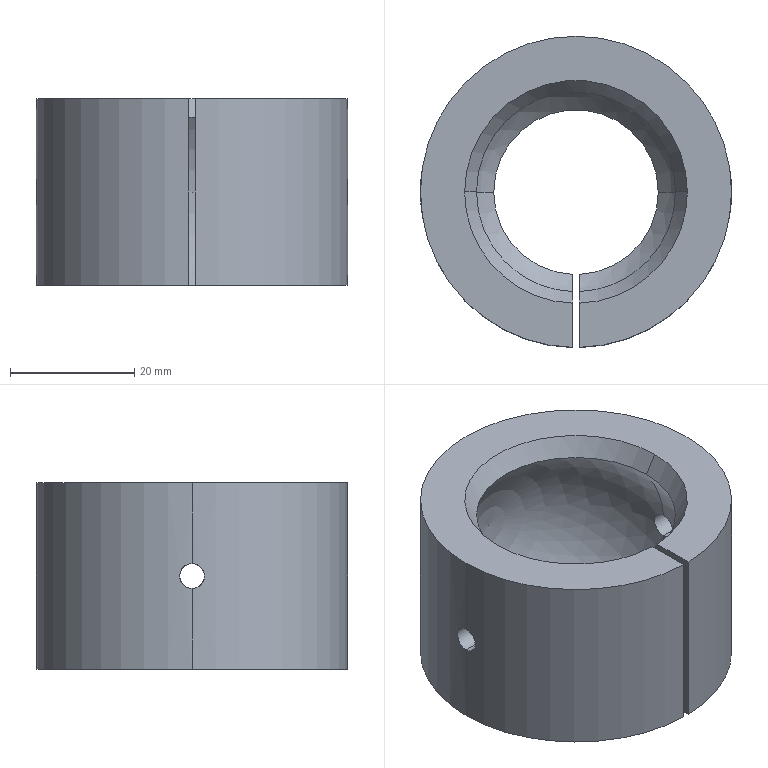Part | SolidWorks | features ICE 2, Revolution 1 | 1 solid | 17 faces | box 50 x 49.995 x 30 mm | volume 27277 mm3 | cylinder 7 | plane 4 | cone 3 | sphere 3 | commonest cylinder face diameters 4 x4 50 x3
STEP:
#1=CARTESIAN_POINT('',(19.9,0.,2.));
#2=VERTEX_POINT('',#1);
#3=CARTESIAN_POINT('',(19.9,0.,-2.));
#4=VERTEX_POINT('',#3);
#5=CARTESIAN_POINT('',(19.9,0.,0.));
#6=DIRECTION('',(1.,0.,0.));
#7=DIRECTION('',(0.,0.,1.));
#8=AXIS2_PLACEMENT_3D('',#5,#6,#7);
#9=CIRCLE('',#8,2.);
#10=EDGE_CURVE('',#2,#4,#9,.T.);
#11=ORIENTED_EDGE('',*,*,#10,.F.);
#12=CARTESIAN_POINT('',(25.,0.,2.));
#13=VERTEX_POINT('',#12);
#14=CARTESIAN_POINT('',(-25.,0.,2.));
#15=DIRECTION('',(1.,0.,0.));
#16=VECTOR('',#15,1000.);
#17=LINE('',#14,#16);
#18=EDGE_CURVE('',#2,#13,#17,.T.);
#19=ORIENTED_EDGE('',*,*,#18,.T.);
#20=CARTESIAN_POINT('',(25.,0.,-2.));
#21=VERTEX_POINT('',#20);
#22=CARTESIAN_POINT('',(25.,0.,-2.));
#23=CARTESIAN_POINT('',(25.,-0.1322,-2.));
#24=CARTESIAN_POINT('',(24.999,-0.2622,-1.987));
#25=CARTESIAN_POINT('',(24.995,-0.5179,-1.936));
#26=CARTESIAN_POINT('',(24.992,-0.6449,-1.898));
#27=CARTESIAN_POINT('',(24.985,-0.8871,-1.797));
#28=CARTESIAN_POINT('',(24.98,-1.002,-1.736));
#29=CARTESIAN_POINT('',(24.97,-1.219,-1.591));
#30=CARTESIAN_POINT('',(24.965,-1.322,-1.506));
#31=CARTESIAN_POINT('',(24.95,-1.599,-1.229));
#32=CARTESIAN_POINT('',(24.939,-1.748,-1.006));
#33=CARTESIAN_POINT('',(24.924,-1.947,-0.525));
#34=CARTESIAN_POINT('',(24.92,-2.,-0.2617));
#35=CARTESIAN_POINT('',(24.92,-2.,0.1298));
#36=CARTESIAN_POINT('',(24.921,-1.987,0.2623));
#37=CARTESIAN_POINT('',(24.925,-1.936,0.5189));
#38=CARTESIAN_POINT('',(24.928,-1.898,0.6436));
#39=CARTESIAN_POINT('',(24.935,-1.798,0.8858));
#40=CARTESIAN_POINT('',(24.94,-1.735,1.003));
#41=CARTESIAN_POINT('',(24.949,-1.59,1.22));
#42=CARTESIAN_POINT('',(24.955,-1.508,1.321));
#43=CARTESIAN_POINT('',(24.965,-1.321,1.507));
#44=CARTESIAN_POINT('',(24.97,-1.22,1.59));
#45=CARTESIAN_POINT('',(24.98,-1.003,1.735));
#46=CARTESIAN_POINT('',(24.985,-0.8865,1.798));
#47=CARTESIAN_POINT('',(24.992,-0.6442,1.898));
#48=CARTESIAN_POINT('',(24.995,-0.5195,1.936));
#49=CARTESIAN_POINT('',(24.999,-0.2632,1.987));
#50=CARTESIAN_POINT('',(25.,-0.1306,2.));
#51=CARTESIAN_POINT('',(25.,0.,2.));
#52=B_SPLINE_CURVE_WITH_KNOTS('',3,(#22,#23,#24,#25,#26,#27,#28,#29,#30,#31,#32,#33,#34,#35,#36,#37,#38,#39,#40,#41,#42,#43,#44,#45,#46,#47,#48,#49,#50,#51),.UNSPECIFIED.,.F.,.F.,(4,2,2,2,2,2,2,2,2,2,2,2,2,2,4),(0.,0.000391,0.0007819,0.001173,0.001564,0.002346,0.003128,0.003519,0.00391,0.004301,0.004692,0.005083,0.005473,0.005864,0.006255),.UNSPECIFIED.);
#53=EDGE_CURVE('',#21,#13,#52,.T.);
#54=ORIENTED_EDGE('',*,*,#53,.F.);
#55=CARTESIAN_POINT('',(-25.,0.,-2.));
#56=DIRECTION('',(1.,0.,0.));
#57=VECTOR('',#56,1000.);
#58=LINE('',#55,#57);
#59=EDGE_CURVE('',#4,#21,#58,.T.);
#60=ORIENTED_EDGE('',*,*,#59,.F.);
#61=EDGE_LOOP('',(#11,#19,#54,#60));
#62=FACE_OUTER_BOUND('',#61,.T.);
#63=CARTESIAN_POINT('',(-25.,0.,0.));
#64=DIRECTION('',(1.,0.,0.));
#65=DIRECTION('',(0.,0.,-1.));
#66=AXIS2_PLACEMENT_3D('',#63,#64,#65);
#67=CYLINDRICAL_SURFACE('',#66,2.);
#68=ADVANCED_FACE('',(#62),#67,.F.);
#69=CARTESIAN_POINT('',(-25.,0.,2.));
#70=VERTEX_POINT('',#69);
#71=CARTESIAN_POINT('',(-25.,0.,-2.));
#72=VERTEX_POINT('',#71);
#73=CARTESIAN_POINT('',(-25.,0.,2.));
#74=CARTESIAN_POINT('',(-25.,-0.2611,2.));
#75=CARTESIAN_POINT('',(-24.996,-0.5242,1.948));
#76=CARTESIAN_POINT('',(-24.981,-1.006,1.748));
#77=CARTESIAN_POINT('',(-24.97,-1.229,1.599));
#78=CARTESIAN_POINT('',(-24.955,-1.505,1.323));
#79=CARTESIAN_POINT('',(-24.949,-1.59,1.22));
#80=CARTESIAN_POINT('',(-24.94,-1.735,1.003));
#81=CARTESIAN_POINT('',(-24.935,-1.797,0.8882));
#82=CARTESIAN_POINT('',(-24.928,-1.897,0.6463));
#83=CARTESIAN_POINT('',(-24.925,-1.936,0.5191));
#84=CARTESIAN_POINT('',(-24.921,-1.987,0.2635));
#85=CARTESIAN_POINT('',(-24.92,-2.,0.1336));
#86=CARTESIAN_POINT('',(-24.92,-2.,-0.1304));
#87=CARTESIAN_POINT('',(-24.921,-1.987,-0.2607));
#88=CARTESIAN_POINT('',(-24.925,-1.937,-0.5164));
#89=CARTESIAN_POINT('',(-24.928,-1.898,-0.6433));
#90=CARTESIAN_POINT('',(-24.935,-1.798,-0.8857));
#91=CARTESIAN_POINT('',(-24.94,-1.737,-1.001));
#92=CARTESIAN_POINT('',(-24.949,-1.592,-1.218));
#93=CARTESIAN_POINT('',(-24.955,-1.507,-1.321));
#94=CARTESIAN_POINT('',(-24.97,-1.231,-1.598));
#95=CARTESIAN_POINT('',(-24.981,-1.008,-1.747));
#96=CARTESIAN_POINT('',(-24.996,-0.527,-1.947));
#97=CARTESIAN_POINT('',(-25.,-0.2643,-2.));
#98=CARTESIAN_POINT('',(-25.,0.,-2.));
#99=B_SPLINE_CURVE_WITH_KNOTS('',3,(#73,#74,#75,#76,#77,#78,#79,#80,#81,#82,#83,#84,#85,#86,#87,#88,#89,#90,#91,#92,#93,#94,#95,#96,#97,#98),.UNSPECIFIED.,.F.,.F.,(4,2,2,2,2,2,2,2,2,2,2,2,4),(0.006255,0.007037,0.007819,0.00821,0.008601,0.008992,0.009382,0.009773,0.01016,0.01056,0.01095,0.01173,0.01251),.UNSPECIFIED.);
#100=EDGE_CURVE('',#70,#72,#99,.T.);
#101=ORIENTED_EDGE('',*,*,#100,.F.);
#102=CARTESIAN_POINT('',(-19.9,0.,2.));
#103=VERTEX_POINT('',#102);
#104=CARTESIAN_POINT('',(-25.,0.,2.));
#105=DIRECTION('',(1.,0.,0.));
#106=VECTOR('',#105,1000.);
#107=LINE('',#104,#106);
#108=EDGE_CURVE('',#70,#103,#107,.T.);
#109=ORIENTED_EDGE('',*,*,#108,.T.);
#110=CARTESIAN_POINT('',(-19.9,0.,-2.));
#111=VERTEX_POINT('',#110);
#112=CARTESIAN_POINT('',(-19.9,0.,0.));
#113=DIRECTION('',(-1.,0.,0.));
#114=DIRECTION('',(0.,0.,-1.));
#115=AXIS2_PLACEMENT_3D('',#112,#113,#114);
#116=CIRCLE('',#115,2.);
#117=EDGE_CURVE('',#111,#103,#116,.T.);
#118=ORIENTED_EDGE('',*,*,#117,.F.);
#119=CARTESIAN_POINT('',(-25.,0.,-2.));
#120=DIRECTION('',(1.,0.,0.));
#121=VECTOR('',#120,1000.);
#122=LINE('',#119,#121);
#123=EDGE_CURVE('',#72,#111,#122,.T.);
#124=ORIENTED_EDGE('',*,*,#123,.F.);
#125=EDGE_LOOP('',(#101,#109,#118,#124));
#126=FACE_OUTER_BOUND('',#125,.T.);
#127=CARTESIAN_POINT('',(-25.,0.,0.));
#128=DIRECTION('',(1.,0.,0.));
#129=DIRECTION('',(0.,0.,-1.));
#130=AXIS2_PLACEMENT_3D('',#127,#128,#129);
#131=CYLINDRICAL_SURFACE('',#130,2.);
#132=ADVANCED_FACE('',(#126),#131,.F.);
#133=CARTESIAN_POINT('',(-0.5,-15.992,12.));
#134=VERTEX_POINT('',#133);
#135=CARTESIAN_POINT('',(-16.,0.,12.));
#136=VERTEX_POINT('',#135);
#137=CARTESIAN_POINT('',(0.,0.,12.));
#138=DIRECTION('',(0.,0.,-1.));
#139=DIRECTION('',(-1.,0.,0.));
#140=AXIS2_PLACEMENT_3D('',#137,#138,#139);
#141=CIRCLE('',#140,16.);
#142=EDGE_CURVE('',#134,#136,#141,.T.);
#143=ORIENTED_EDGE('',*,*,#142,.T.);
#144=CARTESIAN_POINT('',(-17.9,0.,15.));
#145=VERTEX_POINT('',#144);
#146=CARTESIAN_POINT('',(-16.,0.,12.));
#147=DIRECTION('',(-0.5351,0.,0.8448));
#148=VECTOR('',#147,1000.);
#149=LINE('',#146,#148);
#150=EDGE_CURVE('',#136,#145,#149,.T.);
#151=ORIENTED_EDGE('',*,*,#150,.T.);
#152=CARTESIAN_POINT('',(-0.5,-17.893,15.));
#153=VERTEX_POINT('',#152);
#154=CARTESIAN_POINT('',(0.,0.,15.));
#155=DIRECTION('',(0.,0.,-1.));
#156=DIRECTION('',(-1.,0.,0.));
#157=AXIS2_PLACEMENT_3D('',#154,#155,#156);
#158=CIRCLE('',#157,17.9);
#159=EDGE_CURVE('',#153,#145,#158,.T.);
#160=ORIENTED_EDGE('',*,*,#159,.F.);
#161=CARTESIAN_POINT('',(-0.5,-17.893,15.));
#162=CARTESIAN_POINT('',(-0.5,-17.259,14.));
#163=CARTESIAN_POINT('',(-0.5,-16.626,13.));
#164=CARTESIAN_POINT('',(-0.5,-15.992,12.));
#165=B_SPLINE_CURVE_WITH_KNOTS('',3,(#161,#162,#163,#164),.UNSPECIFIED.,.F.,.F.,(4,4),(0.01915,0.0227),.UNSPECIFIED.);
#166=EDGE_CURVE('',#153,#134,#165,.T.);
#167=ORIENTED_EDGE('',*,*,#166,.T.);
#168=EDGE_LOOP('',(#143,#151,#160,#167));
#169=FACE_OUTER_BOUND('',#168,.T.);
#170=CARTESIAN_POINT('',(0.,0.,12.));
#171=DIRECTION('',(0.,0.,1.));
#172=DIRECTION('',(1.,0.,0.));
#173=AXIS2_PLACEMENT_3D('',#170,#171,#172);
#174=CONICAL_SURFACE('',#173,16.,0.5646);
#175=ADVANCED_FACE('',(#169),#174,.F.);
#176=ORIENTED_EDGE('',*,*,#150,.F.);
#177=CARTESIAN_POINT('',(16.,0.,12.));
#178=VERTEX_POINT('',#177);
#179=CARTESIAN_POINT('',(0.,0.,12.));
#180=DIRECTION('',(0.,0.,-1.));
#181=DIRECTION('',(-1.,0.,0.));
#182=AXIS2_PLACEMENT_3D('',#179,#180,#181);
#183=CIRCLE('',#182,16.);
#184=EDGE_CURVE('',#136,#178,#183,.T.);
#185=ORIENTED_EDGE('',*,*,#184,.T.);
#186=CARTESIAN_POINT('',(17.9,0.,15.));
#187=VERTEX_POINT('',#186);
#188=CARTESIAN_POINT('',(16.,0.,12.));
#189=DIRECTION('',(0.5351,0.,0.8448));
#190=VECTOR('',#189,1000.);
#191=LINE('',#188,#190);
#192=EDGE_CURVE('',#178,#187,#191,.T.);
#193=ORIENTED_EDGE('',*,*,#192,.T.);
#194=CARTESIAN_POINT('',(0.,0.,15.));
#195=DIRECTION('',(0.,0.,-1.));
#196=DIRECTION('',(-1.,0.,0.));
#197=AXIS2_PLACEMENT_3D('',#194,#195,#196);
#198=CIRCLE('',#197,17.9);
#199=EDGE_CURVE('',#145,#187,#198,.T.);
#200=ORIENTED_EDGE('',*,*,#199,.F.);
#201=EDGE_LOOP('',(#176,#185,#193,#200));
#202=FACE_OUTER_BOUND('',#201,.T.);
#203=CARTESIAN_POINT('',(0.,0.,12.));
#204=DIRECTION('',(0.,0.,1.));
#205=DIRECTION('',(1.,0.,0.));
#206=AXIS2_PLACEMENT_3D('',#203,#204,#205);
#207=CONICAL_SURFACE('',#206,16.,0.5646);
#208=ADVANCED_FACE('',(#202),#207,.F.);
#209=ORIENTED_EDGE('',*,*,#184,.F.);
#210=CARTESIAN_POINT('',(0.,0.,0.));
#211=DIRECTION('',(0.,-1.,0.));
#212=DIRECTION('',(1.,0.,0.));
#213=AXIS2_PLACEMENT_3D('',#210,#211,#212);
#214=CIRCLE('',#213,20.);
#215=EDGE_CURVE('',#136,#103,#214,.T.);
#216=ORIENTED_EDGE('',*,*,#215,.T.);
#217=CARTESIAN_POINT('',(-19.9,0.,0.));
#218=DIRECTION('',(-1.,0.,0.));
#219=DIRECTION('',(0.,0.,-1.));
#220=AXIS2_PLACEMENT_3D('',#217,#218,#219);
#221=CIRCLE('',#220,2.);
#222=EDGE_CURVE('',#103,#111,#221,.T.);
#223=ORIENTED_EDGE('',*,*,#222,.T.);
#224=CARTESIAN_POINT('',(-13.229,0.,-15.));
#225=VERTEX_POINT('',#224);
#226=CARTESIAN_POINT('',(0.,0.,0.));
#227=DIRECTION('',(0.,-1.,0.));
#228=DIRECTION('',(1.,0.,0.));
#229=AXIS2_PLACEMENT_3D('',#226,#227,#228);
#230=CIRCLE('',#229,20.);
#231=EDGE_CURVE('',#111,#225,#230,.T.);
#232=ORIENTED_EDGE('',*,*,#231,.T.);
#233=CARTESIAN_POINT('',(13.229,0.,-15.));
#234=VERTEX_POINT('',#233);
#235=CARTESIAN_POINT('',(0.,0.,-15.));
#236=DIRECTION('',(0.,0.,-1.));
#237=DIRECTION('',(-1.,0.,0.));
#238=AXIS2_PLACEMENT_3D('',#235,#236,#237);
#239=CIRCLE('',#238,13.229);
#240=EDGE_CURVE('',#225,#234,#239,.T.);
#241=ORIENTED_EDGE('',*,*,#240,.T.);
#242=CARTESIAN_POINT('',(0.,0.,0.));
#243=DIRECTION('',(0.,1.,0.));
#244=DIRECTION('',(0.,0.,1.));
#245=AXIS2_PLACEMENT_3D('',#242,#243,#244);
#246=CIRCLE('',#245,20.);
#247=EDGE_CURVE('',#4,#234,#246,.T.);
#248=ORIENTED_EDGE('',*,*,#247,.F.);
#249=CARTESIAN_POINT('',(19.9,0.,0.));
#250=DIRECTION('',(1.,0.,0.));
#251=DIRECTION('',(0.,0.,1.));
#252=AXIS2_PLACEMENT_3D('',#249,#250,#251);
#253=CIRCLE('',#252,2.);
#254=EDGE_CURVE('',#4,#2,#253,.T.);
#255=ORIENTED_EDGE('',*,*,#254,.T.);
#256=CARTESIAN_POINT('',(0.,0.,0.));
#257=DIRECTION('',(0.,1.,0.));
#258=DIRECTION('',(0.,0.,1.));
#259=AXIS2_PLACEMENT_3D('',#256,#257,#258);
#260=CIRCLE('',#259,20.);
#261=EDGE_CURVE('',#178,#2,#260,.T.);
#262=ORIENTED_EDGE('',*,*,#261,.F.);
#263=EDGE_LOOP('',(#209,#216,#223,#232,#241,#248,#255,#262));
#264=FACE_OUTER_BOUND('',#263,.T.);
#265=CARTESIAN_POINT('',(0.,0.,0.));
#266=DIRECTION('',(0.,-1.,0.));
#267=DIRECTION('',(1.,0.,0.));
#268=AXIS2_PLACEMENT_3D('',#265,#266,#267);
#269=SPHERICAL_SURFACE('',#268,20.);
#270=ADVANCED_FACE('',(#264),#269,.F.);
#271=CARTESIAN_POINT('',(0.5,-15.992,12.));
#272=VERTEX_POINT('',#271);
#273=CARTESIAN_POINT('',(0.,0.,12.));
#274=DIRECTION('',(0.,0.,-1.));
#275=DIRECTION('',(-1.,0.,0.));
#276=AXIS2_PLACEMENT_3D('',#273,#274,#275);
#277=CIRCLE('',#276,16.);
#278=EDGE_CURVE('',#178,#272,#277,.T.);
#279=ORIENTED_EDGE('',*,*,#278,.F.);
#280=ORIENTED_EDGE('',*,*,#261,.T.);
#281=ORIENTED_EDGE('',*,*,#10,.T.);
#282=ORIENTED_EDGE('',*,*,#247,.T.);
#283=CARTESIAN_POINT('',(0.5,-13.219,-15.));
#284=VERTEX_POINT('',#283);
#285=CARTESIAN_POINT('',(0.,0.,-15.));
#286=DIRECTION('',(0.,0.,-1.));
#287=DIRECTION('',(-1.,0.,0.));
#288=AXIS2_PLACEMENT_3D('',#285,#286,#287);
#289=CIRCLE('',#288,13.229);
#290=EDGE_CURVE('',#234,#284,#289,.T.);
#291=ORIENTED_EDGE('',*,*,#290,.T.);
#292=CARTESIAN_POINT('',(0.5,0.,0.));
#293=DIRECTION('',(-1.,0.,0.));
#294=DIRECTION('',(0.,0.,-1.));
#295=AXIS2_PLACEMENT_3D('',#292,#293,#294);
#296=CIRCLE('',#295,19.994);
#297=EDGE_CURVE('',#284,#272,#296,.T.);
#298=ORIENTED_EDGE('',*,*,#297,.T.);
#299=EDGE_LOOP('',(#279,#280,#281,#282,#291,#298));
#300=FACE_OUTER_BOUND('',#299,.T.);
#301=CARTESIAN_POINT('',(0.,0.,0.));
#302=DIRECTION('',(0.,-1.,0.));
#303=DIRECTION('',(1.,0.,0.));
#304=AXIS2_PLACEMENT_3D('',#301,#302,#303);
#305=SPHERICAL_SURFACE('',#304,20.);
#306=ADVANCED_FACE('',(#300),#305,.F.);
#307=CARTESIAN_POINT('',(-25.,0.,15.));
#308=VERTEX_POINT('',#307);
#309=CARTESIAN_POINT('',(25.,0.,15.));
#310=VERTEX_POINT('',#309);
#311=CARTESIAN_POINT('',(0.,0.,15.));
#312=DIRECTION('',(0.,0.,-1.));
#313=DIRECTION('',(-1.,0.,0.));
#314=AXIS2_PLACEMENT_3D('',#311,#312,#313);
#315=CIRCLE('',#314,25.);
#316=EDGE_CURVE('',#308,#310,#315,.T.);
#317=ORIENTED_EDGE('',*,*,#316,.T.);
#318=CARTESIAN_POINT('',(25.,0.,-23.629));
#319=DIRECTION('',(0.,0.,-1.));
#320=VECTOR('',#319,1000.);
#321=LINE('',#318,#320);
#322=EDGE_CURVE('',#310,#13,#321,.T.);
#323=ORIENTED_EDGE('',*,*,#322,.T.);
#324=CARTESIAN_POINT('',(25.,0.,2.));
#325=CARTESIAN_POINT('',(25.,0.2611,2.));
#326=CARTESIAN_POINT('',(24.996,0.5242,1.948));
#327=CARTESIAN_POINT('',(24.981,1.006,1.748));
#328=CARTESIAN_POINT('',(24.97,1.229,1.599));
#329=CARTESIAN_POINT('',(24.955,1.505,1.323));
#330=CARTESIAN_POINT('',(24.949,1.59,1.22));
#331=CARTESIAN_POINT('',(24.94,1.735,1.003));
#332=CARTESIAN_POINT('',(24.935,1.797,0.8882));
#333=CARTESIAN_POINT('',(24.928,1.897,0.6463));
#334=CARTESIAN_POINT('',(24.925,1.936,0.5191));
#335=CARTESIAN_POINT('',(24.921,1.987,0.2635));
#336=CARTESIAN_POINT('',(24.92,2.,0.1336));
#337=CARTESIAN_POINT('',(24.92,2.,-0.1304));
#338=CARTESIAN_POINT('',(24.921,1.987,-0.2607));
#339=CARTESIAN_POINT('',(24.925,1.937,-0.5164));
#340=CARTESIAN_POINT('',(24.928,1.898,-0.6433));
#341=CARTESIAN_POINT('',(24.935,1.798,-0.8857));
#342=CARTESIAN_POINT('',(24.94,1.737,-1.001));
#343=CARTESIAN_POINT('',(24.949,1.592,-1.218));
#344=CARTESIAN_POINT('',(24.955,1.507,-1.321));
#345=CARTESIAN_POINT('',(24.97,1.231,-1.598));
#346=CARTESIAN_POINT('',(24.981,1.008,-1.747));
#347=CARTESIAN_POINT('',(24.996,0.527,-1.947));
#348=CARTESIAN_POINT('',(25.,0.2643,-2.));
#349=CARTESIAN_POINT('',(25.,0.,-2.));
#350=B_SPLINE_CURVE_WITH_KNOTS('',3,(#324,#325,#326,#327,#328,#329,#330,#331,#332,#333,#334,#335,#336,#337,#338,#339,#340,#341,#342,#343,#344,#345,#346,#347,#348,#349),.UNSPECIFIED.,.F.,.F.,(4,2,2,2,2,2,2,2,2,2,2,2,4),(0.006255,0.007037,0.007819,0.00821,0.008601,0.008992,0.009382,0.009773,0.01016,0.01056,0.01095,0.01173,0.01251),.UNSPECIFIED.);
#351=EDGE_CURVE('',#13,#21,#350,.T.);
#352=ORIENTED_EDGE('',*,*,#351,.T.);
#353=CARTESIAN_POINT('',(25.,0.,-15.));
#354=VERTEX_POINT('',#353);
#355=CARTESIAN_POINT('',(25.,0.,-23.629));
#356=DIRECTION('',(0.,0.,-1.));
#357=VECTOR('',#356,1000.);
#358=LINE('',#355,#357);
#359=EDGE_CURVE('',#21,#354,#358,.T.);
#360=ORIENTED_EDGE('',*,*,#359,.T.);
#361=CARTESIAN_POINT('',(-25.,0.,-15.));
#362=VERTEX_POINT('',#361);
#363=CARTESIAN_POINT('',(0.,0.,-15.));
#364=DIRECTION('',(0.,0.,-1.));
#365=DIRECTION('',(-1.,0.,0.));
#366=AXIS2_PLACEMENT_3D('',#363,#364,#365);
#367=CIRCLE('',#366,25.);
#368=EDGE_CURVE('',#362,#354,#367,.T.);
#369=ORIENTED_EDGE('',*,*,#368,.F.);
#370=CARTESIAN_POINT('',(-25.,0.,-23.629));
#371=DIRECTION('',(0.,0.,-1.));
#372=VECTOR('',#371,1000.);
#373=LINE('',#370,#372);
#374=EDGE_CURVE('',#72,#362,#373,.T.);
#375=ORIENTED_EDGE('',*,*,#374,.F.);
#376=CARTESIAN_POINT('',(-25.,0.,-2.));
#377=CARTESIAN_POINT('',(-25.,0.1322,-2.));
#378=CARTESIAN_POINT('',(-24.999,0.2622,-1.987));
#379=CARTESIAN_POINT('',(-24.995,0.5179,-1.936));
#380=CARTESIAN_POINT('',(-24.992,0.6449,-1.898));
#381=CARTESIAN_POINT('',(-24.985,0.8871,-1.797));
#382=CARTESIAN_POINT('',(-24.98,1.002,-1.736));
#383=CARTESIAN_POINT('',(-24.97,1.219,-1.591));
#384=CARTESIAN_POINT('',(-24.965,1.322,-1.506));
#385=CARTESIAN_POINT('',(-24.95,1.599,-1.229));
#386=CARTESIAN_POINT('',(-24.939,1.748,-1.006));
#387=CARTESIAN_POINT('',(-24.924,1.947,-0.525));
#388=CARTESIAN_POINT('',(-24.92,2.,-0.2617));
#389=CARTESIAN_POINT('',(-24.92,2.,0.1298));
#390=CARTESIAN_POINT('',(-24.921,1.987,0.2623));
#391=CARTESIAN_POINT('',(-24.925,1.936,0.5189));
#392=CARTESIAN_POINT('',(-24.928,1.898,0.6436));
#393=CARTESIAN_POINT('',(-24.935,1.798,0.8858));
#394=CARTESIAN_POINT('',(-24.94,1.735,1.003));
#395=CARTESIAN_POINT('',(-24.949,1.59,1.22));
#396=CARTESIAN_POINT('',(-24.955,1.508,1.321));
#397=CARTESIAN_POINT('',(-24.965,1.321,1.507));
#398=CARTESIAN_POINT('',(-24.97,1.22,1.59));
#399=CARTESIAN_POINT('',(-24.98,1.003,1.735));
#400=CARTESIAN_POINT('',(-24.985,0.8865,1.798));
#401=CARTESIAN_POINT('',(-24.992,0.6442,1.898));
#402=CARTESIAN_POINT('',(-24.995,0.5195,1.936));
#403=CARTESIAN_POINT('',(-24.999,0.2632,1.987));
#404=CARTESIAN_POINT('',(-25.,0.1306,2.));
#405=CARTESIAN_POINT('',(-25.,0.,2.));
#406=B_SPLINE_CURVE_WITH_KNOTS('',3,(#376,#377,#378,#379,#380,#381,#382,#383,#384,#385,#386,#387,#388,#389,#390,#391,#392,#393,#394,#395,#396,#397,#398,#399,#400,#401,#402,#403,#404,#405),.UNSPECIFIED.,.F.,.F.,(4,2,2,2,2,2,2,2,2,2,2,2,2,2,4),(0.,0.000391,0.0007819,0.001173,0.001564,0.002346,0.003128,0.003519,0.00391,0.004301,0.004692,0.005083,0.005473,0.005864,0.006255),.UNSPECIFIED.);
#407=EDGE_CURVE('',#72,#70,#406,.T.);
#408=ORIENTED_EDGE('',*,*,#407,.T.);
#409=CARTESIAN_POINT('',(-25.,0.,-23.629));
#410=DIRECTION('',(0.,0.,-1.));
#411=VECTOR('',#410,1000.);
#412=LINE('',#409,#411);
#413=EDGE_CURVE('',#308,#70,#412,.T.);
#414=ORIENTED_EDGE('',*,*,#413,.F.);
#415=EDGE_LOOP('',(#317,#323,#352,#360,#369,#375,#408,#414));
#416=FACE_OUTER_BOUND('',#415,.T.);
#417=CARTESIAN_POINT('',(0.,0.,-23.629));
#418=DIRECTION('',(0.,0.,-1.));
#419=DIRECTION('',(-1.,0.,0.));
#420=AXIS2_PLACEMENT_3D('',#417,#418,#419);
#421=CYLINDRICAL_SURFACE('',#420,25.);
#422=ADVANCED_FACE('',(#416),#421,.T.);
#423=CARTESIAN_POINT('',(-0.5,-24.995,15.));
#424=VERTEX_POINT('',#423);
#425=CARTESIAN_POINT('',(0.,0.,15.));
#426=DIRECTION('',(0.,0.,-1.));
#427=DIRECTION('',(-1.,0.,0.));
#428=AXIS2_PLACEMENT_3D('',#425,#426,#427);
#429=CIRCLE('',#428,25.);
#430=EDGE_CURVE('',#424,#308,#429,.T.);
#431=ORIENTED_EDGE('',*,*,#430,.T.);
#432=ORIENTED_EDGE('',*,*,#413,.T.);
#433=ORIENTED_EDGE('',*,*,#100,.T.);
#434=ORIENTED_EDGE('',*,*,#374,.T.);
#435=CARTESIAN_POINT('',(-0.5,-24.995,-15.));
#436=VERTEX_POINT('',#435);
#437=CARTESIAN_POINT('',(0.,0.,-15.));
#438=DIRECTION('',(0.,0.,-1.));
#439=DIRECTION('',(-1.,0.,0.));
#440=AXIS2_PLACEMENT_3D('',#437,#438,#439);
#441=CIRCLE('',#440,25.);
#442=EDGE_CURVE('',#436,#362,#441,.T.);
#443=ORIENTED_EDGE('',*,*,#442,.F.);
#444=CARTESIAN_POINT('',(-0.5,-24.995,-23.629));
#445=DIRECTION('',(0.,0.,1.));
#446=VECTOR('',#445,1000.);
#447=LINE('',#444,#446);
#448=EDGE_CURVE('',#436,#424,#447,.T.);
#449=ORIENTED_EDGE('',*,*,#448,.T.);
#450=EDGE_LOOP('',(#431,#432,#433,#434,#443,#449));
#451=FACE_OUTER_BOUND('',#450,.T.);
#452=CARTESIAN_POINT('',(0.,0.,-23.629));
#453=DIRECTION('',(0.,0.,-1.));
#454=DIRECTION('',(-1.,0.,0.));
#455=AXIS2_PLACEMENT_3D('',#452,#453,#454);
#456=CYLINDRICAL_SURFACE('',#455,25.);
#457=ADVANCED_FACE('',(#451),#456,.T.);
#458=ORIENTED_EDGE('',*,*,#322,.F.);
#459=CARTESIAN_POINT('',(0.5,-24.995,15.));
#460=VERTEX_POINT('',#459);
#461=CARTESIAN_POINT('',(0.,0.,15.));
#462=DIRECTION('',(0.,0.,-1.));
#463=DIRECTION('',(-1.,0.,0.));
#464=AXIS2_PLACEMENT_3D('',#461,#462,#463);
#465=CIRCLE('',#464,25.);
#466=EDGE_CURVE('',#310,#460,#465,.T.);
#467=ORIENTED_EDGE('',*,*,#466,.T.);
#468=CARTESIAN_POINT('',(0.5,-24.995,-15.));
#469=VERTEX_POINT('',#468);
#470=CARTESIAN_POINT('',(0.5,-24.995,-23.629));
#471=DIRECTION('',(0.,0.,-1.));
#472=VECTOR('',#471,1000.);
#473=LINE('',#470,#472);
#474=EDGE_CURVE('',#460,#469,#473,.T.);
#475=ORIENTED_EDGE('',*,*,#474,.T.);
#476=CARTESIAN_POINT('',(0.,0.,-15.));
#477=DIRECTION('',(0.,0.,-1.));
#478=DIRECTION('',(-1.,0.,0.));
#479=AXIS2_PLACEMENT_3D('',#476,#477,#478);
#480=CIRCLE('',#479,25.);
#481=EDGE_CURVE('',#354,#469,#480,.T.);
#482=ORIENTED_EDGE('',*,*,#481,.F.);
#483=ORIENTED_EDGE('',*,*,#359,.F.);
#484=ORIENTED_EDGE('',*,*,#53,.T.);
#485=EDGE_LOOP('',(#458,#467,#475,#482,#483,#484));
#486=FACE_OUTER_BOUND('',#485,.T.);
#487=CARTESIAN_POINT('',(0.,0.,-23.629));
#488=DIRECTION('',(0.,0.,-1.));
#489=DIRECTION('',(-1.,0.,0.));
#490=AXIS2_PLACEMENT_3D('',#487,#488,#489);
#491=CYLINDRICAL_SURFACE('',#490,25.);
#492=ADVANCED_FACE('',(#486),#491,.T.);
#493=CARTESIAN_POINT('',(-0.5,-13.219,-15.));
#494=VERTEX_POINT('',#493);
#495=CARTESIAN_POINT('',(0.,0.,-15.));
#496=DIRECTION('',(0.,0.,-1.));
#497=DIRECTION('',(-1.,0.,0.));
#498=AXIS2_PLACEMENT_3D('',#495,#496,#497);
#499=CIRCLE('',#498,13.229);
#500=EDGE_CURVE('',#494,#225,#499,.T.);
#501=ORIENTED_EDGE('',*,*,#500,.F.);
#502=CARTESIAN_POINT('',(-0.5,0.,-15.));
#503=DIRECTION('',(0.,-1.,0.));
#504=VECTOR('',#503,1000.);
#505=LINE('',#502,#504);
#506=EDGE_CURVE('',#494,#436,#505,.T.);
#507=ORIENTED_EDGE('',*,*,#506,.T.);
#508=ORIENTED_EDGE('',*,*,#442,.T.);
#509=ORIENTED_EDGE('',*,*,#368,.T.);
#510=ORIENTED_EDGE('',*,*,#481,.T.);
#511=CARTESIAN_POINT('',(0.5,0.,-15.));
#512=DIRECTION('',(0.,1.,0.));
#513=VECTOR('',#512,1000.);
#514=LINE('',#511,#513);
#515=EDGE_CURVE('',#469,#284,#514,.T.);
#516=ORIENTED_EDGE('',*,*,#515,.T.);
#517=ORIENTED_EDGE('',*,*,#290,.F.);
#518=ORIENTED_EDGE('',*,*,#240,.F.);
#519=EDGE_LOOP('',(#501,#507,#508,#509,#510,#516,#517,#518));
#520=FACE_OUTER_BOUND('',#519,.T.);
#521=CARTESIAN_POINT('',(13.229,0.,-15.));
#522=DIRECTION('',(0.,0.,1.));
#523=DIRECTION('',(1.,0.,0.));
#524=AXIS2_PLACEMENT_3D('',#521,#522,#523);
#525=PLANE('',#524);
#526=ADVANCED_FACE('',(#520),#525,.F.);
#527=ORIENTED_EDGE('',*,*,#215,.F.);
#528=ORIENTED_EDGE('',*,*,#142,.F.);
#529=CARTESIAN_POINT('',(-0.5,0.,0.));
#530=DIRECTION('',(1.,0.,0.));
#531=DIRECTION('',(0.,0.,1.));
#532=AXIS2_PLACEMENT_3D('',#529,#530,#531);
#533=CIRCLE('',#532,19.994);
#534=EDGE_CURVE('',#134,#494,#533,.T.);
#535=ORIENTED_EDGE('',*,*,#534,.T.);
#536=ORIENTED_EDGE('',*,*,#500,.T.);
#537=ORIENTED_EDGE('',*,*,#231,.F.);
#538=ORIENTED_EDGE('',*,*,#117,.T.);
#539=EDGE_LOOP('',(#527,#528,#535,#536,#537,#538));
#540=FACE_OUTER_BOUND('',#539,.T.);
#541=CARTESIAN_POINT('',(0.,0.,0.));
#542=DIRECTION('',(0.,-1.,0.));
#543=DIRECTION('',(1.,0.,0.));
#544=AXIS2_PLACEMENT_3D('',#541,#542,#543);
#545=SPHERICAL_SURFACE('',#544,20.);
#546=ADVANCED_FACE('',(#540),#545,.F.);
#547=ORIENTED_EDGE('',*,*,#192,.F.);
#548=ORIENTED_EDGE('',*,*,#278,.T.);
#549=CARTESIAN_POINT('',(0.5,-17.893,15.));
#550=VERTEX_POINT('',#549);
#551=CARTESIAN_POINT('',(0.5,-15.992,12.));
#552=CARTESIAN_POINT('',(0.5,-16.187,12.307));
#553=CARTESIAN_POINT('',(0.5,-16.381,12.614));
#554=CARTESIAN_POINT('',(0.5,-16.576,12.921));
#555=CARTESIAN_POINT('',(0.5,-17.015,13.614));
#556=CARTESIAN_POINT('',(0.5,-17.454,14.307));
#557=CARTESIAN_POINT('',(0.5,-17.893,15.));
#558=B_SPLINE_CURVE_WITH_KNOTS('',3,(#551,#552,#553,#554,#555,#556,#557),.UNSPECIFIED.,.F.,.F.,(4,3,4),(0.02052,0.02161,0.02407),.UNSPECIFIED.);
#559=EDGE_CURVE('',#272,#550,#558,.T.);
#560=ORIENTED_EDGE('',*,*,#559,.T.);
#561=CARTESIAN_POINT('',(0.,0.,15.));
#562=DIRECTION('',(0.,0.,-1.));
#563=DIRECTION('',(-1.,0.,0.));
#564=AXIS2_PLACEMENT_3D('',#561,#562,#563);
#565=CIRCLE('',#564,17.9);
#566=EDGE_CURVE('',#187,#550,#565,.T.);
#567=ORIENTED_EDGE('',*,*,#566,.F.);
#568=EDGE_LOOP('',(#547,#548,#560,#567));
#569=FACE_OUTER_BOUND('',#568,.T.);
#570=CARTESIAN_POINT('',(0.,0.,12.));
#571=DIRECTION('',(0.,0.,1.));
#572=DIRECTION('',(1.,0.,0.));
#573=AXIS2_PLACEMENT_3D('',#570,#571,#572);
#574=CONICAL_SURFACE('',#573,16.,0.5646);
#575=ADVANCED_FACE('',(#569),#574,.F.);
#576=ORIENTED_EDGE('',*,*,#430,.F.);
#577=CARTESIAN_POINT('',(-0.5,0.,15.));
#578=DIRECTION('',(0.,1.,0.));
#579=VECTOR('',#578,1000.);
#580=LINE('',#577,#579);
#581=EDGE_CURVE('',#424,#153,#580,.T.);
#582=ORIENTED_EDGE('',*,*,#581,.T.);
#583=ORIENTED_EDGE('',*,*,#159,.T.);
#584=ORIENTED_EDGE('',*,*,#199,.T.);
#585=ORIENTED_EDGE('',*,*,#566,.T.);
#586=CARTESIAN_POINT('',(0.5,0.,15.));
#587=DIRECTION('',(0.,-1.,0.));
#588=VECTOR('',#587,1000.);
#589=LINE('',#586,#588);
#590=EDGE_CURVE('',#550,#460,#589,.T.);
#591=ORIENTED_EDGE('',*,*,#590,.T.);
#592=ORIENTED_EDGE('',*,*,#466,.F.);
#593=ORIENTED_EDGE('',*,*,#316,.F.);
#594=EDGE_LOOP('',(#576,#582,#583,#584,#585,#591,#592,#593));
#595=FACE_OUTER_BOUND('',#594,.T.);
#596=CARTESIAN_POINT('',(17.9,0.,15.));
#597=DIRECTION('',(0.,0.,-1.));
#598=DIRECTION('',(-1.,0.,0.));
#599=AXIS2_PLACEMENT_3D('',#596,#597,#598);
#600=PLANE('',#599);
#601=ADVANCED_FACE('',(#595),#600,.F.);
#602=ORIENTED_EDGE('',*,*,#590,.F.);
#603=ORIENTED_EDGE('',*,*,#559,.F.);
#604=ORIENTED_EDGE('',*,*,#297,.F.);
#605=ORIENTED_EDGE('',*,*,#515,.F.);
#606=ORIENTED_EDGE('',*,*,#474,.F.);
#607=EDGE_LOOP('',(#602,#603,#604,#605,#606));
#608=FACE_OUTER_BOUND('',#607,.T.);
#609=CARTESIAN_POINT('',(0.5,-25.,-17.5));
#610=DIRECTION('',(1.,0.,0.));
#611=DIRECTION('',(0.,0.,-1.));
#612=AXIS2_PLACEMENT_3D('',#609,#610,#611);
#613=PLANE('',#612);
#614=ADVANCED_FACE('',(#608),#613,.F.);
#615=ORIENTED_EDGE('',*,*,#506,.F.);
#616=ORIENTED_EDGE('',*,*,#534,.F.);
#617=ORIENTED_EDGE('',*,*,#166,.F.);
#618=ORIENTED_EDGE('',*,*,#581,.F.);
#619=ORIENTED_EDGE('',*,*,#448,.F.);
#620=EDGE_LOOP('',(#615,#616,#617,#618,#619));
#621=FACE_OUTER_BOUND('',#620,.T.);
#622=CARTESIAN_POINT('',(-0.5,-25.,-17.5));
#623=DIRECTION('',(-1.,0.,0.));
#624=DIRECTION('',(0.,0.,1.));
#625=AXIS2_PLACEMENT_3D('',#622,#623,#624);
#626=PLANE('',#625);
#627=ADVANCED_FACE('',(#621),#626,.F.);
#628=ORIENTED_EDGE('',*,*,#108,.F.);
#629=ORIENTED_EDGE('',*,*,#407,.F.);
#630=ORIENTED_EDGE('',*,*,#123,.T.);
#631=ORIENTED_EDGE('',*,*,#222,.F.);
#632=EDGE_LOOP('',(#628,#629,#630,#631));
#633=FACE_OUTER_BOUND('',#632,.T.);
#634=CARTESIAN_POINT('',(-25.,0.,0.));
#635=DIRECTION('',(1.,0.,0.));
#636=DIRECTION('',(0.,0.,-1.));
#637=AXIS2_PLACEMENT_3D('',#634,#635,#636);
#638=CYLINDRICAL_SURFACE('',#637,2.);
#639=ADVANCED_FACE('',(#633),#638,.F.);
#640=ORIENTED_EDGE('',*,*,#18,.F.);
#641=ORIENTED_EDGE('',*,*,#254,.F.);
#642=ORIENTED_EDGE('',*,*,#59,.T.);
#643=ORIENTED_EDGE('',*,*,#351,.F.);
#644=EDGE_LOOP('',(#640,#641,#642,#643));
#645=FACE_OUTER_BOUND('',#644,.T.);
#646=CARTESIAN_POINT('',(-25.,0.,0.));
#647=DIRECTION('',(1.,0.,0.));
#648=DIRECTION('',(0.,0.,-1.));
#649=AXIS2_PLACEMENT_3D('',#646,#647,#648);
#650=CYLINDRICAL_SURFACE('',#649,2.);
#651=ADVANCED_FACE('',(#645),#650,.F.);
#652=CLOSED_SHELL('',(#68,#132,#175,#208,#270,#306,#422,#457,#492,#526,#546,#575,#601,#614,#627,#639,#651));
#653=MANIFOLD_SOLID_BREP('',#652);
#654=CARTESIAN_POINT('',(0.,0.,0.));
#655=DIRECTION('',(0.,0.,1.));
#656=DIRECTION('',(1.,0.,0.));
#657=AXIS2_PLACEMENT_3D('',#654,#655,#656);
#658=(LENGTH_UNIT()NAMED_UNIT(*)SI_UNIT(.MILLI.,.METRE.));
#659=UNCERTAINTY_MEASURE_WITH_UNIT(LENGTH_MEASURE(0.00001),#658,'','');
#660=(NAMED_UNIT(*)PLANE_ANGLE_UNIT()SI_UNIT($,.RADIAN.));
#661=(NAMED_UNIT(*)SI_UNIT($,.STERADIAN.)SOLID_ANGLE_UNIT());
#662=(GEOMETRIC_REPRESENTATION_CONTEXT(3)GLOBAL_UNCERTAINTY_ASSIGNED_CONTEXT((#659))GLOBAL_UNIT_ASSIGNED_CONTEXT((#658,#660,#661))REPRESENTATION_CONTEXT('',''));
#663=ADVANCED_BREP_SHAPE_REPRESENTATION('',(#653,#657),#662);